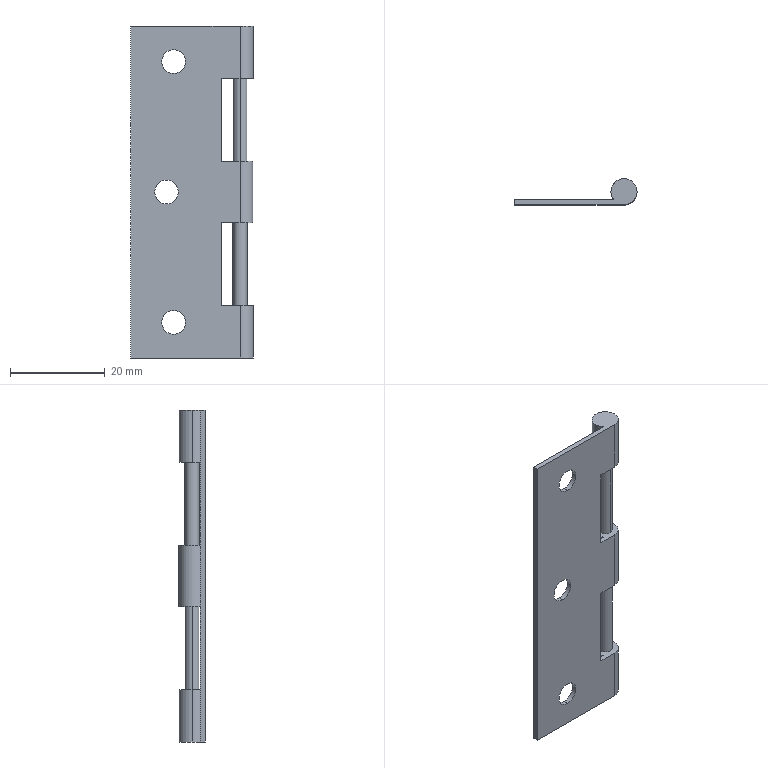Part | STEP file | 70 hinge-1 | 1 solid | 29 faces | box 25.75 x 5.5 x 70 mm | volume 2438 mm3 | cylinder 18 | plane 11 | commonest cylinder face diameters 5.5 x8 5 x6 3 x4